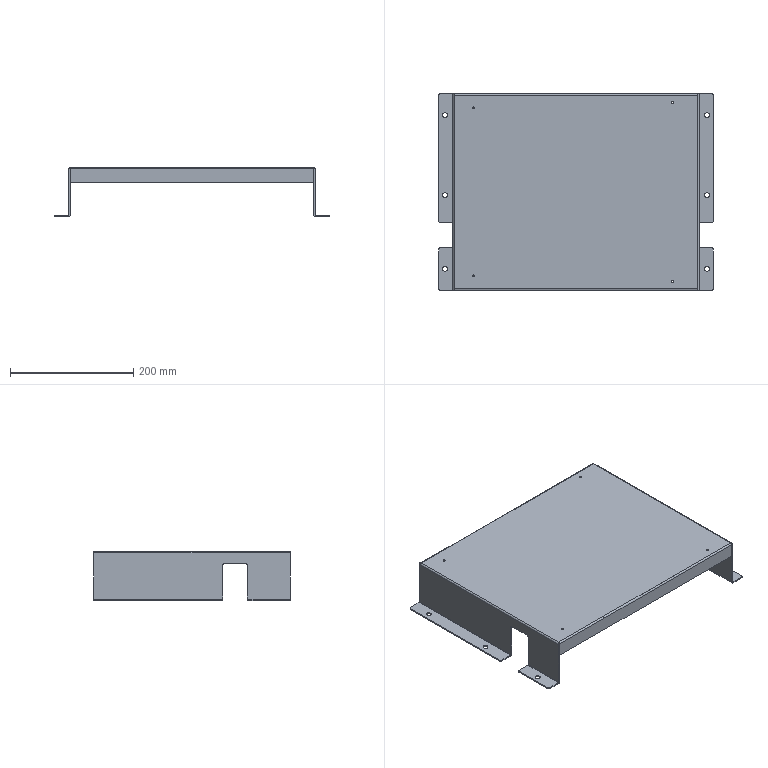Part | STEP file | TJ-DHQM-003-016 | 1 solid | 114 faces | box 446 x 320 x 80 mm | volume 405095 mm3 | plane 66 | cylinder 48 | commonest cylinder face diameters 5 x20 8 x12 1 x8 3.3 x8